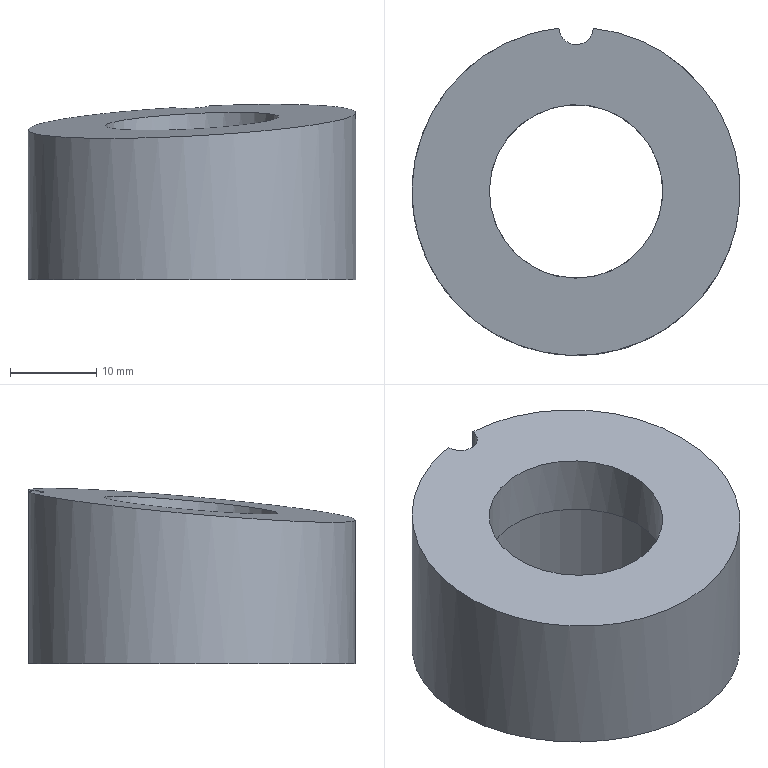Part | NX | features EKSD 38-20-20.10 2 | 1 solid | 7 faces | box 38 x 37.895 x 20.31 mm | volume 11878 mm3 | cylinder 4 | plane 3 | commonest cylinder face diameters 4 x1 20.1 x1 26.6 x1 38 x1
STEP:
#1=CARTESIAN_POINT('',(-192.893,7.418,-24.));
#2=VERTEX_POINT('',#1);
#3=CARTESIAN_POINT('',(-188.899,7.418,-24.));
#4=VERTEX_POINT('',#3);
#5=CARTESIAN_POINT('',(-190.896,7.523,-24.));
#6=DIRECTION('',(0.,0.,-1.));
#7=DIRECTION('',(-1.,0.,0.));
#8=AXIS2_PLACEMENT_3D('',#5,#6,#7);
#9=CIRCLE('',#8,2.);
#10=EDGE_CURVE('',#2,#4,#9,.F.);
#11=ORIENTED_EDGE('',*,*,#10,.T.);
#12=CARTESIAN_POINT('',(-190.896,-11.477,-24.));
#13=DIRECTION('',(0.,0.,-1.));
#14=DIRECTION('',(-1.,0.,0.));
#15=AXIS2_PLACEMENT_3D('',#12,#13,#14);
#16=CIRCLE('',#15,19.);
#17=EDGE_CURVE('',#2,#4,#16,.F.);
#18=ORIENTED_EDGE('',*,*,#17,.F.);
#19=EDGE_LOOP('',(#11,#18));
#20=FACE_BOUND('',#19,.T.);
#21=CARTESIAN_POINT('',(-204.196,-11.477,-24.));
#22=VERTEX_POINT('',#21);
#23=CARTESIAN_POINT('',(-190.896,-11.477,-24.));
#24=DIRECTION('',(0.,0.,-1.));
#25=DIRECTION('',(-1.,0.,0.));
#26=AXIS2_PLACEMENT_3D('',#23,#24,#25);
#27=CIRCLE('',#26,13.3);
#28=EDGE_CURVE('',#22,#22,#27,.T.);
#29=ORIENTED_EDGE('',*,*,#28,.F.);
#30=EDGE_LOOP('',(#29));
#31=FACE_BOUND('',#30,.T.);
#32=CARTESIAN_POINT('',(-190.896,-11.477,-24.));
#33=DIRECTION('',(0.,0.,-1.));
#34=DIRECTION('',(-1.,0.,0.));
#35=AXIS2_PLACEMENT_3D('',#32,#33,#34);
#36=PLANE('',#35);
#37=ADVANCED_FACE('',(#20,#31),#36,.T.);
#38=CARTESIAN_POINT('',(-188.899,7.418,-3.864));
#39=VERTEX_POINT('',#38);
#40=CARTESIAN_POINT('',(-192.893,7.418,-4.073));
#41=VERTEX_POINT('',#40);
#42=CARTESIAN_POINT('',(-190.896,7.523,-3.959));
#43=DIRECTION('',(0.05204,0.08903,-0.9947));
#44=DIRECTION('',(-0.502,-0.8587,-0.1031));
#45=AXIS2_PLACEMENT_3D('',#42,#43,#44);
#46=ELLIPSE('',#45,2.011,2.);
#47=EDGE_CURVE('',#39,#41,#46,.T.);
#48=ORIENTED_EDGE('',*,*,#47,.T.);
#49=CARTESIAN_POINT('',(-190.896,-11.477,-5.66));
#50=DIRECTION('',(0.05204,0.08903,-0.9947));
#51=DIRECTION('',(-0.502,-0.8587,-0.1031));
#52=AXIS2_PLACEMENT_3D('',#49,#50,#51);
#53=ELLIPSE('',#52,19.102,19.);
#54=EDGE_CURVE('',#39,#41,#53,.T.);
#55=ORIENTED_EDGE('',*,*,#54,.F.);
#56=EDGE_LOOP('',(#48,#55));
#57=FACE_BOUND('',#56,.T.);
#58=CARTESIAN_POINT('',(-195.968,-20.153,-6.702));
#59=VERTEX_POINT('',#58);
#60=CARTESIAN_POINT('',(-190.896,-11.477,-5.66));
#61=DIRECTION('',(0.05204,0.08903,-0.9947));
#62=DIRECTION('',(-0.502,-0.8587,-0.1031));
#63=AXIS2_PLACEMENT_3D('',#60,#61,#62);
#64=ELLIPSE('',#63,10.104,10.05);
#65=EDGE_CURVE('',#59,#59,#64,.F.);
#66=ORIENTED_EDGE('',*,*,#65,.F.);
#67=EDGE_LOOP('',(#66));
#68=FACE_BOUND('',#67,.T.);
#69=CARTESIAN_POINT('',(-99.272,-11.445,-0.8629));
#70=DIRECTION('',(0.05204,0.08903,-0.9947));
#71=DIRECTION('',(0.005002,-0.996,-0.08889));
#72=AXIS2_PLACEMENT_3D('',#69,#70,#71);
#73=PLANE('',#72);
#74=ADVANCED_FACE('',(#57,#68),#73,.F.);
#75=CARTESIAN_POINT('',(-188.899,7.418,-13.5));
#76=DIRECTION('',(0.,0.,-1.));
#77=VECTOR('',#76,1000.);
#78=LINE('',#75,#77);
#79=EDGE_CURVE('',#39,#4,#78,.T.);
#80=ORIENTED_EDGE('',*,*,#79,.F.);
#81=ORIENTED_EDGE('',*,*,#54,.T.);
#82=CARTESIAN_POINT('',(-192.893,7.418,-13.5));
#83=DIRECTION('',(0.,0.,-1.));
#84=VECTOR('',#83,1000.);
#85=LINE('',#82,#84);
#86=EDGE_CURVE('',#2,#41,#85,.F.);
#87=ORIENTED_EDGE('',*,*,#86,.F.);
#88=ORIENTED_EDGE('',*,*,#17,.T.);
#89=EDGE_LOOP('',(#80,#81,#87,#88));
#90=FACE_BOUND('',#89,.T.);
#91=CARTESIAN_POINT('',(-190.896,-11.477,-3.5));
#92=DIRECTION('',(0.,0.,-1.));
#93=DIRECTION('',(-1.,0.,0.));
#94=AXIS2_PLACEMENT_3D('',#91,#92,#93);
#95=CYLINDRICAL_SURFACE('',#94,19.);
#96=ADVANCED_FACE('',(#90),#95,.T.);
#97=CARTESIAN_POINT('',(-180.846,-11.477,-11.5));
#98=VERTEX_POINT('',#97);
#99=CARTESIAN_POINT('',(-190.896,-11.477,-11.5));
#100=DIRECTION('',(0.,0.,1.));
#101=DIRECTION('',(1.,0.,0.));
#102=AXIS2_PLACEMENT_3D('',#99,#100,#101);
#103=CIRCLE('',#102,10.05);
#104=EDGE_CURVE('',#98,#98,#103,.F.);
#105=ORIENTED_EDGE('',*,*,#104,.T.);
#106=EDGE_LOOP('',(#105));
#107=FACE_BOUND('',#106,.T.);
#108=ORIENTED_EDGE('',*,*,#65,.T.);
#109=EDGE_LOOP('',(#108));
#110=FACE_BOUND('',#109,.T.);
#111=CARTESIAN_POINT('',(-190.896,-11.477,-2.5));
#112=DIRECTION('',(0.,0.,-1.));
#113=DIRECTION('',(-1.,0.,0.));
#114=AXIS2_PLACEMENT_3D('',#111,#112,#113);
#115=CYLINDRICAL_SURFACE('',#114,10.05);
#116=ADVANCED_FACE('',(#107,#110),#115,.F.);
#117=CARTESIAN_POINT('',(-204.196,-11.477,-11.5));
#118=VERTEX_POINT('',#117);
#119=CARTESIAN_POINT('',(-190.896,-11.477,-11.5));
#120=DIRECTION('',(0.,0.,-1.));
#121=DIRECTION('',(-1.,0.,0.));
#122=AXIS2_PLACEMENT_3D('',#119,#120,#121);
#123=CIRCLE('',#122,13.3);
#124=EDGE_CURVE('',#118,#118,#123,.T.);
#125=ORIENTED_EDGE('',*,*,#124,.T.);
#126=EDGE_LOOP('',(#125));
#127=FACE_BOUND('',#126,.T.);
#128=ORIENTED_EDGE('',*,*,#104,.F.);
#129=EDGE_LOOP('',(#128));
#130=FACE_BOUND('',#129,.T.);
#131=CARTESIAN_POINT('',(-190.896,-11.477,-11.5));
#132=DIRECTION('',(0.,0.,1.));
#133=DIRECTION('',(1.,0.,0.));
#134=AXIS2_PLACEMENT_3D('',#131,#132,#133);
#135=PLANE('',#134);
#136=ADVANCED_FACE('',(#127,#130),#135,.F.);
#137=ORIENTED_EDGE('',*,*,#28,.T.);
#138=EDGE_LOOP('',(#137));
#139=FACE_BOUND('',#138,.T.);
#140=ORIENTED_EDGE('',*,*,#124,.F.);
#141=EDGE_LOOP('',(#140));
#142=FACE_BOUND('',#141,.T.);
#143=CARTESIAN_POINT('',(-190.896,-11.477,-11.5));
#144=DIRECTION('',(0.,0.,-1.));
#145=DIRECTION('',(-1.,0.,0.));
#146=AXIS2_PLACEMENT_3D('',#143,#144,#145);
#147=CYLINDRICAL_SURFACE('',#146,13.3);
#148=ADVANCED_FACE('',(#139,#142),#147,.F.);
#149=ORIENTED_EDGE('',*,*,#79,.T.);
#150=ORIENTED_EDGE('',*,*,#10,.F.);
#151=ORIENTED_EDGE('',*,*,#86,.T.);
#152=ORIENTED_EDGE('',*,*,#47,.F.);
#153=EDGE_LOOP('',(#149,#150,#151,#152));
#154=FACE_BOUND('',#153,.T.);
#155=CARTESIAN_POINT('',(-190.896,7.523,-3.5));
#156=DIRECTION('',(0.,0.,-1.));
#157=DIRECTION('',(-1.,0.,0.));
#158=AXIS2_PLACEMENT_3D('',#155,#156,#157);
#159=CYLINDRICAL_SURFACE('',#158,2.);
#160=ADVANCED_FACE('',(#154),#159,.F.);
#161=CLOSED_SHELL('',(#37,#74,#96,#116,#136,#148,#160));
#162=MANIFOLD_SOLID_BREP('',#161);
#163=(LENGTH_UNIT()NAMED_UNIT(*)SI_UNIT(.MILLI.,.METRE.));
#164=UNCERTAINTY_MEASURE_WITH_UNIT(LENGTH_MEASURE(0.00001),#163,'','');
#165=(NAMED_UNIT(*)PLANE_ANGLE_UNIT()SI_UNIT($,.RADIAN.));
#166=(NAMED_UNIT(*)SI_UNIT($,.STERADIAN.)SOLID_ANGLE_UNIT());
#167=(GEOMETRIC_REPRESENTATION_CONTEXT(3)GLOBAL_UNCERTAINTY_ASSIGNED_CONTEXT((#164))GLOBAL_UNIT_ASSIGNED_CONTEXT((#163,#165,#166))REPRESENTATION_CONTEXT('',''));
#168=ADVANCED_BREP_SHAPE_REPRESENTATION('',(#162),#167);